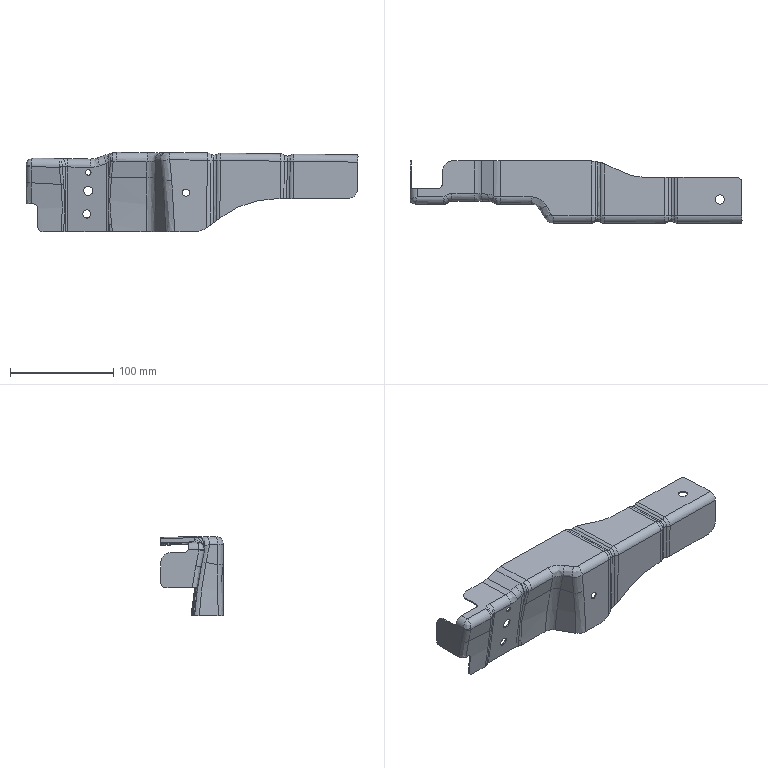Part | 1 solid | 254 faces | box 321.5 x 60.379 x 76.639 mm | volume 41441 mm3 | spline 146 | cylinder 68 | plane 36 | other 4 | commonest cylinder face diameters 10 x15 12.4 x10 11.6 x9 14 x9 9 x4 7.6 x3